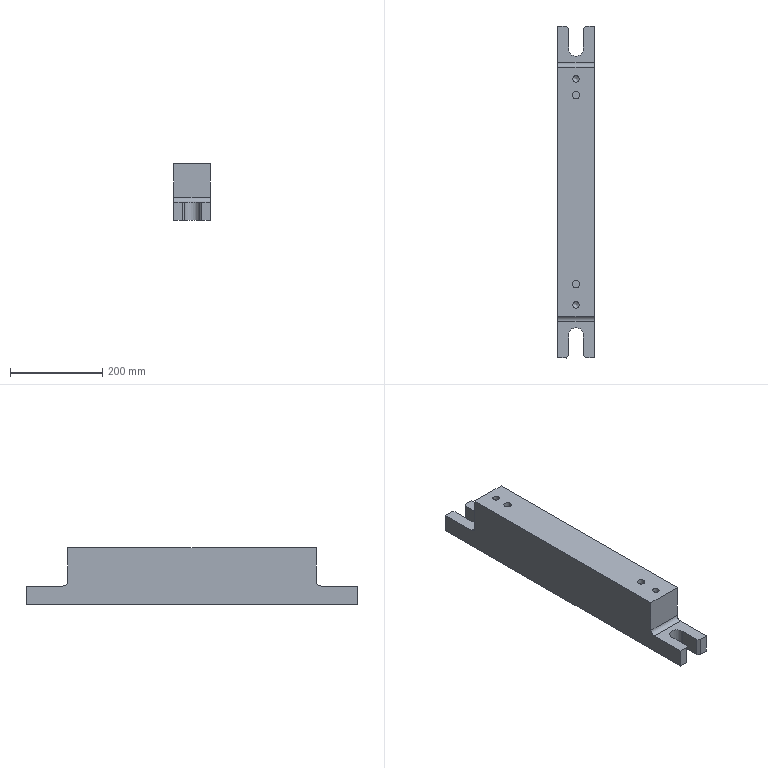Part | NX | features LIN_SOLID_COLOR 2 | 1 solid | 32 faces | box 80 x 720 x 123.5 mm | volume 5723645 mm3 | plane 22 | cylinder 8 | cone 2 | commonest cylinder face diameters 14 x2 16.002 x2 20 x2 32 x2
STEP:
#1=CARTESIAN_POINT('',(866.,-270.,-180.));
#2=VERTEX_POINT('',#1);
#3=CARTESIAN_POINT('',(786.,-270.,-180.));
#4=VERTEX_POINT('',#3);
#5=CARTESIAN_POINT('',(786.,-270.,-180.));
#6=DIRECTION('',(1.,0.,0.));
#7=VECTOR('',#6,1000.);
#8=LINE('',#5,#7);
#9=EDGE_CURVE('',#2,#4,#8,.F.);
#10=ORIENTED_EDGE('',*,*,#9,.F.);
#11=CARTESIAN_POINT('',(866.,-270.,-106.5));
#12=VERTEX_POINT('',#11);
#13=CARTESIAN_POINT('',(866.,-270.,-101.5));
#14=DIRECTION('',(0.,0.,-1.));
#15=VECTOR('',#14,1000.);
#16=LINE('',#13,#15);
#17=EDGE_CURVE('',#2,#12,#16,.F.);
#18=ORIENTED_EDGE('',*,*,#17,.T.);
#19=CARTESIAN_POINT('',(786.,-270.,-106.5));
#20=VERTEX_POINT('',#19);
#21=CARTESIAN_POINT('',(76.,-270.,-106.5));
#22=DIRECTION('',(1.,0.,0.));
#23=VECTOR('',#22,1000.);
#24=LINE('',#21,#23);
#25=EDGE_CURVE('',#12,#20,#24,.F.);
#26=ORIENTED_EDGE('',*,*,#25,.T.);
#27=CARTESIAN_POINT('',(786.,-270.,-101.5));
#28=DIRECTION('',(0.,0.,-1.));
#29=VECTOR('',#28,1000.);
#30=LINE('',#27,#29);
#31=EDGE_CURVE('',#4,#20,#30,.F.);
#32=ORIENTED_EDGE('',*,*,#31,.F.);
#33=EDGE_LOOP('',(#10,#18,#26,#32));
#34=FACE_BOUND('',#33,.T.);
#35=CARTESIAN_POINT('',(806.,-270.,-101.5));
#36=DIRECTION('',(0.,-1.,0.));
#37=DIRECTION('',(0.,0.,1.));
#38=AXIS2_PLACEMENT_3D('',#35,#36,#37);
#39=PLANE('',#38);
#40=ADVANCED_FACE('',(#34),#39,.T.);
#41=CARTESIAN_POINT('',(805.,-360.,-230.));
#42=VERTEX_POINT('',#41);
#43=CARTESIAN_POINT('',(786.,-360.,-230.));
#44=VERTEX_POINT('',#43);
#45=CARTESIAN_POINT('',(116.,-360.,-230.));
#46=DIRECTION('',(-1.,0.,0.));
#47=VECTOR('',#46,1000.);
#48=LINE('',#45,#47);
#49=EDGE_CURVE('',#42,#44,#48,.T.);
#50=ORIENTED_EDGE('',*,*,#49,.T.);
#51=CARTESIAN_POINT('',(786.,360.,-230.));
#52=VERTEX_POINT('',#51);
#53=CARTESIAN_POINT('',(786.,0.,-230.));
#54=DIRECTION('',(0.,-1.,0.));
#55=VECTOR('',#54,1000.);
#56=LINE('',#53,#55);
#57=EDGE_CURVE('',#52,#44,#56,.T.);
#58=ORIENTED_EDGE('',*,*,#57,.F.);
#59=CARTESIAN_POINT('',(805.,360.,-230.));
#60=VERTEX_POINT('',#59);
#61=CARTESIAN_POINT('',(116.,360.,-230.));
#62=DIRECTION('',(-1.,0.,0.));
#63=VECTOR('',#62,1000.);
#64=LINE('',#61,#63);
#65=EDGE_CURVE('',#60,#52,#64,.T.);
#66=ORIENTED_EDGE('',*,*,#65,.F.);
#67=CARTESIAN_POINT('',(810.,355.,-230.));
#68=VERTEX_POINT('',#67);
#69=CARTESIAN_POINT('',(126696.583,-125531.583,-230.));
#70=DIRECTION('',(0.7071,-0.7071,0.));
#71=VECTOR('',#70,1000.);
#72=LINE('',#69,#71);
#73=EDGE_CURVE('',#60,#68,#72,.T.);
#74=ORIENTED_EDGE('',*,*,#73,.T.);
#75=CARTESIAN_POINT('',(810.,310.,-230.));
#76=VERTEX_POINT('',#75);
#77=CARTESIAN_POINT('',(810.,1858.277,-230.));
#78=DIRECTION('',(0.,1.,0.));
#79=VECTOR('',#78,1000.);
#80=LINE('',#77,#79);
#81=EDGE_CURVE('',#76,#68,#80,.T.);
#82=ORIENTED_EDGE('',*,*,#81,.F.);
#83=CARTESIAN_POINT('',(842.,310.,-230.));
#84=VERTEX_POINT('',#83);
#85=CARTESIAN_POINT('',(826.,310.,-230.));
#86=DIRECTION('',(0.,0.,-1.));
#87=DIRECTION('',(1.,0.,0.));
#88=AXIS2_PLACEMENT_3D('',#85,#86,#87);
#89=CIRCLE('',#88,16.);
#90=EDGE_CURVE('',#84,#76,#89,.T.);
#91=ORIENTED_EDGE('',*,*,#90,.F.);
#92=CARTESIAN_POINT('',(842.,355.,-230.));
#93=VERTEX_POINT('',#92);
#94=CARTESIAN_POINT('',(842.,1858.277,-230.));
#95=DIRECTION('',(0.,-1.,0.));
#96=VECTOR('',#95,1000.);
#97=LINE('',#94,#96);
#98=EDGE_CURVE('',#93,#84,#97,.T.);
#99=ORIENTED_EDGE('',*,*,#98,.F.);
#100=CARTESIAN_POINT('',(847.,360.,-230.));
#101=VERTEX_POINT('',#100);
#102=CARTESIAN_POINT('',(128215.859,127728.859,-230.));
#103=DIRECTION('',(0.7071,0.7071,0.));
#104=VECTOR('',#103,1000.);
#105=LINE('',#102,#104);
#106=EDGE_CURVE('',#93,#101,#105,.T.);
#107=ORIENTED_EDGE('',*,*,#106,.T.);
#108=CARTESIAN_POINT('',(866.,360.,-230.));
#109=VERTEX_POINT('',#108);
#110=CARTESIAN_POINT('',(116.,360.,-230.));
#111=DIRECTION('',(-1.,0.,0.));
#112=VECTOR('',#111,1000.);
#113=LINE('',#110,#112);
#114=EDGE_CURVE('',#109,#101,#113,.T.);
#115=ORIENTED_EDGE('',*,*,#114,.F.);
#116=CARTESIAN_POINT('',(866.,-360.,-230.));
#117=VERTEX_POINT('',#116);
#118=CARTESIAN_POINT('',(866.,0.,-230.));
#119=DIRECTION('',(0.,-1.,0.));
#120=VECTOR('',#119,1000.);
#121=LINE('',#118,#120);
#122=EDGE_CURVE('',#109,#117,#121,.T.);
#123=ORIENTED_EDGE('',*,*,#122,.T.);
#124=CARTESIAN_POINT('',(847.,-360.,-230.));
#125=VERTEX_POINT('',#124);
#126=CARTESIAN_POINT('',(116.,-360.,-230.));
#127=DIRECTION('',(-1.,0.,0.));
#128=VECTOR('',#127,1000.);
#129=LINE('',#126,#128);
#130=EDGE_CURVE('',#117,#125,#129,.T.);
#131=ORIENTED_EDGE('',*,*,#130,.T.);
#132=CARTESIAN_POINT('',(842.,-355.,-230.));
#133=VERTEX_POINT('',#132);
#134=CARTESIAN_POINT('',(128215.859,-127728.859,-230.));
#135=DIRECTION('',(0.7071,-0.7071,0.));
#136=VECTOR('',#135,1000.);
#137=LINE('',#134,#136);
#138=EDGE_CURVE('',#133,#125,#137,.T.);
#139=ORIENTED_EDGE('',*,*,#138,.F.);
#140=CARTESIAN_POINT('',(842.,-310.,-230.));
#141=VERTEX_POINT('',#140);
#142=CARTESIAN_POINT('',(842.,-1858.277,-230.));
#143=DIRECTION('',(0.,1.,0.));
#144=VECTOR('',#143,1000.);
#145=LINE('',#142,#144);
#146=EDGE_CURVE('',#133,#141,#145,.T.);
#147=ORIENTED_EDGE('',*,*,#146,.T.);
#148=CARTESIAN_POINT('',(810.,-310.,-230.));
#149=VERTEX_POINT('',#148);
#150=CARTESIAN_POINT('',(826.,-310.,-230.));
#151=DIRECTION('',(0.,0.,1.));
#152=DIRECTION('',(1.,0.,0.));
#153=AXIS2_PLACEMENT_3D('',#150,#151,#152);
#154=CIRCLE('',#153,16.);
#155=EDGE_CURVE('',#141,#149,#154,.T.);
#156=ORIENTED_EDGE('',*,*,#155,.T.);
#157=CARTESIAN_POINT('',(810.,-355.,-230.));
#158=VERTEX_POINT('',#157);
#159=CARTESIAN_POINT('',(810.,-1858.277,-230.));
#160=DIRECTION('',(0.,-1.,0.));
#161=VECTOR('',#160,1000.);
#162=LINE('',#159,#161);
#163=EDGE_CURVE('',#149,#158,#162,.T.);
#164=ORIENTED_EDGE('',*,*,#163,.T.);
#165=CARTESIAN_POINT('',(126696.583,125531.583,-230.));
#166=DIRECTION('',(0.7071,0.7071,0.));
#167=VECTOR('',#166,1000.);
#168=LINE('',#165,#167);
#169=EDGE_CURVE('',#42,#158,#168,.T.);
#170=ORIENTED_EDGE('',*,*,#169,.F.);
#171=EDGE_LOOP('',(#50,#58,#66,#74,#82,#91,#99,#107,#115,#123,#131,#139,#147,#156,#164,#170));
#172=FACE_BOUND('',#171,.T.);
#173=CARTESIAN_POINT('',(666.,0.,-230.));
#174=DIRECTION('',(0.,0.,1.));
#175=DIRECTION('',(-1.,0.,0.));
#176=AXIS2_PLACEMENT_3D('',#173,#174,#175);
#177=PLANE('',#176);
#178=ADVANCED_FACE('',(#172),#177,.F.);
#179=CARTESIAN_POINT('',(866.,270.,-106.5));
#180=VERTEX_POINT('',#179);
#181=CARTESIAN_POINT('',(866.,0.,-106.5));
#182=DIRECTION('',(0.,1.,0.));
#183=VECTOR('',#182,1000.);
#184=LINE('',#181,#183);
#185=EDGE_CURVE('',#12,#180,#184,.T.);
#186=ORIENTED_EDGE('',*,*,#185,.T.);
#187=CARTESIAN_POINT('',(786.,270.,-106.5));
#188=VERTEX_POINT('',#187);
#189=CARTESIAN_POINT('',(806.,270.,-106.5));
#190=DIRECTION('',(-1.,0.,0.));
#191=VECTOR('',#190,1000.);
#192=LINE('',#189,#191);
#193=EDGE_CURVE('',#180,#188,#192,.T.);
#194=ORIENTED_EDGE('',*,*,#193,.T.);
#195=CARTESIAN_POINT('',(786.,0.,-106.5));
#196=DIRECTION('',(0.,1.,0.));
#197=VECTOR('',#196,1000.);
#198=LINE('',#195,#197);
#199=EDGE_CURVE('',#20,#188,#198,.T.);
#200=ORIENTED_EDGE('',*,*,#199,.F.);
#201=ORIENTED_EDGE('',*,*,#25,.F.);
#202=EDGE_LOOP('',(#186,#194,#200,#201));
#203=FACE_BOUND('',#202,.T.);
#204=CARTESIAN_POINT('',(817.999,210.,-106.5));
#205=VERTEX_POINT('',#204);
#206=CARTESIAN_POINT('',(826.,210.,-106.5));
#207=DIRECTION('',(0.,0.,-1.));
#208=DIRECTION('',(-1.,0.,0.));
#209=AXIS2_PLACEMENT_3D('',#206,#207,#208);
#210=CIRCLE('',#209,8.001);
#211=EDGE_CURVE('',#205,#205,#210,.T.);
#212=ORIENTED_EDGE('',*,*,#211,.T.);
#213=EDGE_LOOP('',(#212));
#214=FACE_BOUND('',#213,.T.);
#215=CARTESIAN_POINT('',(819.,-245.,-106.5));
#216=VERTEX_POINT('',#215);
#217=CARTESIAN_POINT('',(826.,-245.,-106.5));
#218=DIRECTION('',(0.,0.,-1.));
#219=DIRECTION('',(-1.,0.,0.));
#220=AXIS2_PLACEMENT_3D('',#217,#218,#219);
#221=CIRCLE('',#220,7.);
#222=EDGE_CURVE('',#216,#216,#221,.T.);
#223=ORIENTED_EDGE('',*,*,#222,.T.);
#224=EDGE_LOOP('',(#223));
#225=FACE_BOUND('',#224,.T.);
#226=CARTESIAN_POINT('',(819.,245.,-106.5));
#227=VERTEX_POINT('',#226);
#228=CARTESIAN_POINT('',(826.,245.,-106.5));
#229=DIRECTION('',(0.,0.,-1.));
#230=DIRECTION('',(-1.,0.,0.));
#231=AXIS2_PLACEMENT_3D('',#228,#229,#230);
#232=CIRCLE('',#231,7.);
#233=EDGE_CURVE('',#227,#227,#232,.T.);
#234=ORIENTED_EDGE('',*,*,#233,.T.);
#235=EDGE_LOOP('',(#234));
#236=FACE_BOUND('',#235,.T.);
#237=CARTESIAN_POINT('',(817.999,-200.,-106.5));
#238=VERTEX_POINT('',#237);
#239=CARTESIAN_POINT('',(826.,-200.,-106.5));
#240=DIRECTION('',(0.,0.,-1.));
#241=DIRECTION('',(-1.,0.,0.));
#242=AXIS2_PLACEMENT_3D('',#239,#240,#241);
#243=CIRCLE('',#242,8.001);
#244=EDGE_CURVE('',#238,#238,#243,.F.);
#245=ORIENTED_EDGE('',*,*,#244,.F.);
#246=EDGE_LOOP('',(#245));
#247=FACE_BOUND('',#246,.T.);
#248=CARTESIAN_POINT('',(76.,0.,-106.5));
#249=DIRECTION('',(0.,0.,-1.));
#250=DIRECTION('',(1.,0.,0.));
#251=AXIS2_PLACEMENT_3D('',#248,#249,#250);
#252=PLANE('',#251);
#253=ADVANCED_FACE('',(#203,#214,#225,#236,#247),#252,.F.);
#254=CARTESIAN_POINT('',(866.,270.,-180.));
#255=VERTEX_POINT('',#254);
#256=CARTESIAN_POINT('',(866.,270.,-101.5));
#257=DIRECTION('',(0.,0.,1.));
#258=VECTOR('',#257,1000.);
#259=LINE('',#256,#258);
#260=EDGE_CURVE('',#255,#180,#259,.T.);
#261=ORIENTED_EDGE('',*,*,#260,.F.);
#262=CARTESIAN_POINT('',(786.,270.,-180.));
#263=VERTEX_POINT('',#262);
#264=CARTESIAN_POINT('',(786.,270.,-180.));
#265=DIRECTION('',(1.,0.,0.));
#266=VECTOR('',#265,1000.);
#267=LINE('',#264,#266);
#268=EDGE_CURVE('',#255,#263,#267,.F.);
#269=ORIENTED_EDGE('',*,*,#268,.T.);
#270=CARTESIAN_POINT('',(786.,270.,-101.5));
#271=DIRECTION('',(0.,0.,1.));
#272=VECTOR('',#271,1000.);
#273=LINE('',#270,#272);
#274=EDGE_CURVE('',#263,#188,#273,.T.);
#275=ORIENTED_EDGE('',*,*,#274,.T.);
#276=ORIENTED_EDGE('',*,*,#193,.F.);
#277=EDGE_LOOP('',(#261,#269,#275,#276));
#278=FACE_BOUND('',#277,.T.);
#279=CARTESIAN_POINT('',(806.,270.,-101.5));
#280=DIRECTION('',(0.,-1.,0.));
#281=DIRECTION('',(0.,0.,1.));
#282=AXIS2_PLACEMENT_3D('',#279,#280,#281);
#283=PLANE('',#282);
#284=ADVANCED_FACE('',(#278),#283,.F.);
#285=ORIENTED_EDGE('',*,*,#199,.T.);
#286=ORIENTED_EDGE('',*,*,#274,.F.);
#287=CARTESIAN_POINT('',(786.,280.,-190.));
#288=VERTEX_POINT('',#287);
#289=CARTESIAN_POINT('',(786.,280.,-180.));
#290=DIRECTION('',(1.,0.,0.));
#291=DIRECTION('',(0.,0.,1.));
#292=AXIS2_PLACEMENT_3D('',#289,#290,#291);
#293=CIRCLE('',#292,10.);
#294=EDGE_CURVE('',#263,#288,#293,.T.);
#295=ORIENTED_EDGE('',*,*,#294,.T.);
#296=CARTESIAN_POINT('',(786.,360.,-190.));
#297=VERTEX_POINT('',#296);
#298=CARTESIAN_POINT('',(786.,320.,-190.));
#299=DIRECTION('',(0.,1.,0.));
#300=VECTOR('',#299,1000.);
#301=LINE('',#298,#300);
#302=EDGE_CURVE('',#288,#297,#301,.T.);
#303=ORIENTED_EDGE('',*,*,#302,.T.);
#304=CARTESIAN_POINT('',(786.,360.,-131.5));
#305=DIRECTION('',(0.,0.,1.));
#306=VECTOR('',#305,1000.);
#307=LINE('',#304,#306);
#308=EDGE_CURVE('',#52,#297,#307,.T.);
#309=ORIENTED_EDGE('',*,*,#308,.F.);
#310=ORIENTED_EDGE('',*,*,#57,.T.);
#311=CARTESIAN_POINT('',(786.,-360.,-190.));
#312=VERTEX_POINT('',#311);
#313=CARTESIAN_POINT('',(786.,-360.,-131.5));
#314=DIRECTION('',(0.,0.,1.));
#315=VECTOR('',#314,1000.);
#316=LINE('',#313,#315);
#317=EDGE_CURVE('',#44,#312,#316,.T.);
#318=ORIENTED_EDGE('',*,*,#317,.T.);
#319=CARTESIAN_POINT('',(786.,-280.,-190.));
#320=VERTEX_POINT('',#319);
#321=CARTESIAN_POINT('',(786.,-320.,-190.));
#322=DIRECTION('',(0.,-1.,0.));
#323=VECTOR('',#322,1000.);
#324=LINE('',#321,#323);
#325=EDGE_CURVE('',#320,#312,#324,.T.);
#326=ORIENTED_EDGE('',*,*,#325,.F.);
#327=CARTESIAN_POINT('',(786.,-280.,-180.));
#328=DIRECTION('',(-1.,0.,0.));
#329=DIRECTION('',(0.,0.,1.));
#330=AXIS2_PLACEMENT_3D('',#327,#328,#329);
#331=CIRCLE('',#330,10.);
#332=EDGE_CURVE('',#4,#320,#331,.T.);
#333=ORIENTED_EDGE('',*,*,#332,.F.);
#334=ORIENTED_EDGE('',*,*,#31,.T.);
#335=EDGE_LOOP('',(#285,#286,#295,#303,#309,#310,#318,#326,#333,#334));
#336=FACE_BOUND('',#335,.T.);
#337=CARTESIAN_POINT('',(786.,0.,-101.5));
#338=DIRECTION('',(1.,0.,0.));
#339=DIRECTION('',(0.,0.,1.));
#340=AXIS2_PLACEMENT_3D('',#337,#338,#339);
#341=PLANE('',#340);
#342=ADVANCED_FACE('',(#336),#341,.F.);
#343=CARTESIAN_POINT('',(866.,-360.,-190.));
#344=VERTEX_POINT('',#343);
#345=CARTESIAN_POINT('',(866.,-360.,-111.5));
#346=DIRECTION('',(0.,0.,1.));
#347=VECTOR('',#346,1000.);
#348=LINE('',#345,#347);
#349=EDGE_CURVE('',#117,#344,#348,.T.);
#350=ORIENTED_EDGE('',*,*,#349,.F.);
#351=ORIENTED_EDGE('',*,*,#122,.F.);
#352=CARTESIAN_POINT('',(866.,360.,-190.));
#353=VERTEX_POINT('',#352);
#354=CARTESIAN_POINT('',(866.,360.,-111.5));
#355=DIRECTION('',(0.,0.,1.));
#356=VECTOR('',#355,1000.);
#357=LINE('',#354,#356);
#358=EDGE_CURVE('',#109,#353,#357,.T.);
#359=ORIENTED_EDGE('',*,*,#358,.T.);
#360=CARTESIAN_POINT('',(866.,280.,-190.));
#361=VERTEX_POINT('',#360);
#362=CARTESIAN_POINT('',(866.,10.,-190.));
#363=DIRECTION('',(0.,-1.,0.));
#364=VECTOR('',#363,1000.);
#365=LINE('',#362,#364);
#366=EDGE_CURVE('',#353,#361,#365,.T.);
#367=ORIENTED_EDGE('',*,*,#366,.T.);
#368=CARTESIAN_POINT('',(866.,280.,-180.));
#369=DIRECTION('',(1.,0.,0.));
#370=DIRECTION('',(0.,0.,1.));
#371=AXIS2_PLACEMENT_3D('',#368,#369,#370);
#372=CIRCLE('',#371,10.);
#373=EDGE_CURVE('',#361,#255,#372,.F.);
#374=ORIENTED_EDGE('',*,*,#373,.T.);
#375=ORIENTED_EDGE('',*,*,#260,.T.);
#376=ORIENTED_EDGE('',*,*,#185,.F.);
#377=ORIENTED_EDGE('',*,*,#17,.F.);
#378=CARTESIAN_POINT('',(866.,-280.,-190.));
#379=VERTEX_POINT('',#378);
#380=CARTESIAN_POINT('',(866.,-280.,-180.));
#381=DIRECTION('',(-1.,0.,0.));
#382=DIRECTION('',(0.,0.,1.));
#383=AXIS2_PLACEMENT_3D('',#380,#381,#382);
#384=CIRCLE('',#383,10.);
#385=EDGE_CURVE('',#379,#2,#384,.F.);
#386=ORIENTED_EDGE('',*,*,#385,.F.);
#387=CARTESIAN_POINT('',(866.,-10.,-190.));
#388=DIRECTION('',(0.,1.,0.));
#389=VECTOR('',#388,1000.);
#390=LINE('',#387,#389);
#391=EDGE_CURVE('',#344,#379,#390,.T.);
#392=ORIENTED_EDGE('',*,*,#391,.F.);
#393=EDGE_LOOP('',(#350,#351,#359,#367,#374,#375,#376,#377,#386,#392));
#394=FACE_BOUND('',#393,.T.);
#395=CARTESIAN_POINT('',(866.,0.,-101.5));
#396=DIRECTION('',(1.,0.,0.));
#397=DIRECTION('',(0.,0.,1.));
#398=AXIS2_PLACEMENT_3D('',#395,#396,#397);
#399=PLANE('',#398);
#400=ADVANCED_FACE('',(#394),#399,.T.);
#401=CARTESIAN_POINT('',(833.,-245.,-146.5));
#402=VERTEX_POINT('',#401);
#403=CARTESIAN_POINT('',(826.,-245.,-146.5));
#404=DIRECTION('',(0.,0.,1.));
#405=DIRECTION('',(1.,0.,0.));
#406=AXIS2_PLACEMENT_3D('',#403,#404,#405);
#407=CIRCLE('',#406,7.);
#408=EDGE_CURVE('',#402,#402,#407,.T.);
#409=ORIENTED_EDGE('',*,*,#408,.F.);
#410=EDGE_LOOP('',(#409));
#411=FACE_BOUND('',#410,.T.);
#412=ORIENTED_EDGE('',*,*,#222,.F.);
#413=EDGE_LOOP('',(#412));
#414=FACE_BOUND('',#413,.T.);
#415=CARTESIAN_POINT('',(826.,-245.,-106.4));
#416=DIRECTION('',(0.,0.,-1.));
#417=DIRECTION('',(1.,0.,0.));
#418=AXIS2_PLACEMENT_3D('',#415,#416,#417);
#419=CYLINDRICAL_SURFACE('',#418,7.);
#420=ADVANCED_FACE('',(#411,#414),#419,.F.);
#421=ORIENTED_EDGE('',*,*,#408,.T.);
#422=EDGE_LOOP('',(#421));
#423=FACE_BOUND('',#422,.T.);
#424=CARTESIAN_POINT('',(826.,-245.,-150.541));
#425=VERTEX_POINT('',#424);
#426=VERTEX_LOOP('',#425);
#427=FACE_BOUND('',#426,.T.);
#428=CARTESIAN_POINT('',(826.,-245.,-150.541));
#429=DIRECTION('',(0.,0.,1.));
#430=DIRECTION('',(1.,0.,0.));
#431=AXIS2_PLACEMENT_3D('',#428,#429,#430);
#432=CONICAL_SURFACE('',#431,0.,1.047);
#433=ADVANCED_FACE('',(#423,#427),#432,.F.);
#434=CARTESIAN_POINT('',(833.,245.,-146.5));
#435=VERTEX_POINT('',#434);
#436=CARTESIAN_POINT('',(826.,245.,-146.5));
#437=DIRECTION('',(0.,0.,1.));
#438=DIRECTION('',(1.,0.,0.));
#439=AXIS2_PLACEMENT_3D('',#436,#437,#438);
#440=CIRCLE('',#439,7.);
#441=EDGE_CURVE('',#435,#435,#440,.T.);
#442=ORIENTED_EDGE('',*,*,#441,.F.);
#443=EDGE_LOOP('',(#442));
#444=FACE_BOUND('',#443,.T.);
#445=ORIENTED_EDGE('',*,*,#233,.F.);
#446=EDGE_LOOP('',(#445));
#447=FACE_BOUND('',#446,.T.);
#448=CARTESIAN_POINT('',(826.,245.,-106.4));
#449=DIRECTION('',(0.,0.,-1.));
#450=DIRECTION('',(1.,0.,0.));
#451=AXIS2_PLACEMENT_3D('',#448,#449,#450);
#452=CYLINDRICAL_SURFACE('',#451,7.);
#453=ADVANCED_FACE('',(#444,#447),#452,.F.);
#454=ORIENTED_EDGE('',*,*,#441,.T.);
#455=EDGE_LOOP('',(#454));
#456=FACE_BOUND('',#455,.T.);
#457=CARTESIAN_POINT('',(826.,245.,-150.541));
#458=VERTEX_POINT('',#457);
#459=VERTEX_LOOP('',#458);
#460=FACE_BOUND('',#459,.T.);
#461=CARTESIAN_POINT('',(826.,245.,-150.541));
#462=DIRECTION('',(0.,0.,1.));
#463=DIRECTION('',(1.,0.,0.));
#464=AXIS2_PLACEMENT_3D('',#461,#462,#463);
#465=CONICAL_SURFACE('',#464,0.,1.047);
#466=ADVANCED_FACE('',(#456,#460),#465,.F.);
#467=CARTESIAN_POINT('',(834.001,-200.,-146.5));
#468=VERTEX_POINT('',#467);
#469=CARTESIAN_POINT('',(826.,-200.,-146.5));
#470=DIRECTION('',(0.,0.,1.));
#471=DIRECTION('',(1.,0.,0.));
#472=AXIS2_PLACEMENT_3D('',#469,#470,#471);
#473=CIRCLE('',#472,8.001);
#474=EDGE_CURVE('',#468,#468,#473,.T.);
#475=ORIENTED_EDGE('',*,*,#474,.F.);
#476=EDGE_LOOP('',(#475));
#477=FACE_BOUND('',#476,.T.);
#478=ORIENTED_EDGE('',*,*,#244,.T.);
#479=EDGE_LOOP('',(#478));
#480=FACE_BOUND('',#479,.T.);
#481=CARTESIAN_POINT('',(826.,-200.,-304.5));
#482=DIRECTION('',(0.,0.,1.));
#483=DIRECTION('',(1.,0.,0.));
#484=AXIS2_PLACEMENT_3D('',#481,#482,#483);
#485=CYLINDRICAL_SURFACE('',#484,8.001);
#486=ADVANCED_FACE('',(#477,#480),#485,.F.);
#487=CARTESIAN_POINT('',(834.001,210.,-146.5));
#488=VERTEX_POINT('',#487);
#489=CARTESIAN_POINT('',(826.,210.,-146.5));
#490=DIRECTION('',(0.,0.,1.));
#491=DIRECTION('',(1.,0.,0.));
#492=AXIS2_PLACEMENT_3D('',#489,#490,#491);
#493=CIRCLE('',#492,8.001);
#494=EDGE_CURVE('',#488,#488,#493,.T.);
#495=ORIENTED_EDGE('',*,*,#494,.F.);
#496=EDGE_LOOP('',(#495));
#497=FACE_BOUND('',#496,.T.);
#498=ORIENTED_EDGE('',*,*,#211,.F.);
#499=EDGE_LOOP('',(#498));
#500=FACE_BOUND('',#499,.T.);
#501=CARTESIAN_POINT('',(826.,210.,-304.5));
#502=DIRECTION('',(0.,0.,1.));
#503=DIRECTION('',(1.,0.,0.));
#504=AXIS2_PLACEMENT_3D('',#501,#502,#503);
#505=CYLINDRICAL_SURFACE('',#504,8.001);
#506=ADVANCED_FACE('',(#497,#500),#505,.F.);
#507=ORIENTED_EDGE('',*,*,#130,.F.);
#508=ORIENTED_EDGE('',*,*,#349,.T.);
#509=CARTESIAN_POINT('',(847.,-360.,-190.));
#510=VERTEX_POINT('',#509);
#511=CARTESIAN_POINT('',(116.,-360.,-190.));
#512=DIRECTION('',(1.,0.,0.));
#513=VECTOR('',#512,1000.);
#514=LINE('',#511,#513);
#515=EDGE_CURVE('',#510,#344,#514,.T.);
#516=ORIENTED_EDGE('',*,*,#515,.F.);
#517=CARTESIAN_POINT('',(847.,-360.,-200.));
#518=DIRECTION('',(0.,0.,1.));
#519=VECTOR('',#518,1000.);
#520=LINE('',#517,#519);
#521=EDGE_CURVE('',#125,#510,#520,.T.);
#522=ORIENTED_EDGE('',*,*,#521,.F.);
#523=EDGE_LOOP('',(#507,#508,#516,#522));
#524=FACE_BOUND('',#523,.T.);
#525=CARTESIAN_POINT('',(116.,-360.,-131.5));
#526=DIRECTION('',(0.,-1.,0.));
#527=DIRECTION('',(0.,0.,-1.));
#528=AXIS2_PLACEMENT_3D('',#525,#526,#527);
#529=PLANE('',#528);
#530=ADVANCED_FACE('',(#524),#529,.T.);
#531=ORIENTED_EDGE('',*,*,#138,.T.);
#532=ORIENTED_EDGE('',*,*,#521,.T.);
#533=CARTESIAN_POINT('',(842.,-355.,-190.));
#534=VERTEX_POINT('',#533);
#535=CARTESIAN_POINT('',(616.5,-129.5,-190.));
#536=DIRECTION('',(-0.7071,0.7071,0.));
#537=VECTOR('',#536,1000.);
#538=LINE('',#535,#537);
#539=EDGE_CURVE('',#510,#534,#538,.T.);
#540=ORIENTED_EDGE('',*,*,#539,.T.);
#541=CARTESIAN_POINT('',(842.,-355.,-230.));
#542=DIRECTION('',(0.,0.,-1.));
#543=VECTOR('',#542,1000.);
#544=LINE('',#541,#543);
#545=EDGE_CURVE('',#534,#133,#544,.T.);
#546=ORIENTED_EDGE('',*,*,#545,.T.);
#547=EDGE_LOOP('',(#531,#532,#540,#546));
#548=FACE_BOUND('',#547,.T.);
#549=CARTESIAN_POINT('',(847.,-360.,-131.5));
#550=DIRECTION('',(-0.7071,-0.7071,0.));
#551=DIRECTION('',(0.,0.,-1.));
#552=AXIS2_PLACEMENT_3D('',#549,#550,#551);
#553=PLANE('',#552);
#554=ADVANCED_FACE('',(#548),#553,.T.);
#555=CARTESIAN_POINT('',(842.,-310.,-190.));
#556=VERTEX_POINT('',#555);
#557=CARTESIAN_POINT('',(842.,-30.,-190.));
#558=DIRECTION('',(0.,-1.,0.));
#559=VECTOR('',#558,1000.);
#560=LINE('',#557,#559);
#561=EDGE_CURVE('',#556,#534,#560,.T.);
#562=ORIENTED_EDGE('',*,*,#561,.F.);
#563=CARTESIAN_POINT('',(842.,-310.,-305.));
#564=DIRECTION('',(0.,0.,1.));
#565=VECTOR('',#564,1000.);
#566=LINE('',#563,#565);
#567=EDGE_CURVE('',#556,#141,#566,.F.);
#568=ORIENTED_EDGE('',*,*,#567,.T.);
#569=ORIENTED_EDGE('',*,*,#146,.F.);
#570=ORIENTED_EDGE('',*,*,#545,.F.);
#571=EDGE_LOOP('',(#562,#568,#569,#570));
#572=FACE_BOUND('',#571,.T.);
#573=CARTESIAN_POINT('',(842.,-60.,-305.));
#574=DIRECTION('',(1.,0.,0.));
#575=DIRECTION('',(0.,0.,1.));
#576=AXIS2_PLACEMENT_3D('',#573,#574,#575);
#577=PLANE('',#576);
#578=ADVANCED_FACE('',(#572),#577,.F.);
#579=CARTESIAN_POINT('',(810.,-310.,-190.));
#580=VERTEX_POINT('',#579);
#581=CARTESIAN_POINT('',(826.,-310.,-190.));
#582=DIRECTION('',(0.,0.,-1.));
#583=DIRECTION('',(-1.,0.,0.));
#584=AXIS2_PLACEMENT_3D('',#581,#582,#583);
#585=CIRCLE('',#584,16.);
#586=EDGE_CURVE('',#580,#556,#585,.T.);
#587=ORIENTED_EDGE('',*,*,#586,.F.);
#588=CARTESIAN_POINT('',(810.,-310.,-305.));
#589=DIRECTION('',(0.,0.,-1.));
#590=VECTOR('',#589,1000.);
#591=LINE('',#588,#590);
#592=EDGE_CURVE('',#149,#580,#591,.F.);
#593=ORIENTED_EDGE('',*,*,#592,.F.);
#594=ORIENTED_EDGE('',*,*,#155,.F.);
#595=ORIENTED_EDGE('',*,*,#567,.F.);
#596=EDGE_LOOP('',(#587,#593,#594,#595));
#597=FACE_BOUND('',#596,.T.);
#598=CARTESIAN_POINT('',(826.,-310.,-155.));
#599=DIRECTION('',(0.,0.,-1.));
#600=DIRECTION('',(1.,0.,0.));
#601=AXIS2_PLACEMENT_3D('',#598,#599,#600);
#602=CYLINDRICAL_SURFACE('',#601,16.);
#603=ADVANCED_FACE('',(#597),#602,.F.);
#604=ORIENTED_EDGE('',*,*,#163,.F.);
#605=ORIENTED_EDGE('',*,*,#592,.T.);
#606=CARTESIAN_POINT('',(810.,-355.,-190.));
#607=VERTEX_POINT('',#606);
#608=CARTESIAN_POINT('',(810.,-30.,-190.));
#609=DIRECTION('',(0.,1.,0.));
#610=VECTOR('',#609,1000.);
#611=LINE('',#608,#610);
#612=EDGE_CURVE('',#607,#580,#611,.T.);
#613=ORIENTED_EDGE('',*,*,#612,.F.);
#614=CARTESIAN_POINT('',(810.,-355.,-200.));
#615=DIRECTION('',(0.,0.,1.));
#616=VECTOR('',#615,1000.);
#617=LINE('',#614,#616);
#618=EDGE_CURVE('',#158,#607,#617,.T.);
#619=ORIENTED_EDGE('',*,*,#618,.F.);
#620=EDGE_LOOP('',(#604,#605,#613,#619));
#621=FACE_BOUND('',#620,.T.);
#622=CARTESIAN_POINT('',(810.,-60.,-305.));
#623=DIRECTION('',(-1.,0.,0.));
#624=DIRECTION('',(0.,0.,-1.));
#625=AXIS2_PLACEMENT_3D('',#622,#623,#624);
#626=PLANE('',#625);
#627=ADVANCED_FACE('',(#621),#626,.F.);
#628=ORIENTED_EDGE('',*,*,#169,.T.);
#629=ORIENTED_EDGE('',*,*,#618,.T.);
#630=CARTESIAN_POINT('',(805.,-360.,-190.));
#631=VERTEX_POINT('',#630);
#632=CARTESIAN_POINT('',(925.5,-239.5,-190.));
#633=DIRECTION('',(-0.7071,-0.7071,0.));
#634=VECTOR('',#633,1000.);
#635=LINE('',#632,#634);
#636=EDGE_CURVE('',#607,#631,#635,.T.);
#637=ORIENTED_EDGE('',*,*,#636,.T.);
#638=CARTESIAN_POINT('',(805.,-360.,-230.));
#639=DIRECTION('',(0.,0.,-1.));
#640=VECTOR('',#639,1000.);
#641=LINE('',#638,#640);
#642=EDGE_CURVE('',#631,#42,#641,.T.);
#643=ORIENTED_EDGE('',*,*,#642,.T.);
#644=EDGE_LOOP('',(#628,#629,#637,#643));
#645=FACE_BOUND('',#644,.T.);
#646=CARTESIAN_POINT('',(810.,-355.,-305.));
#647=DIRECTION('',(0.7071,-0.7071,0.));
#648=DIRECTION('',(0.,0.,-1.));
#649=AXIS2_PLACEMENT_3D('',#646,#647,#648);
#650=PLANE('',#649);
#651=ADVANCED_FACE('',(#645),#650,.T.);
#652=ORIENTED_EDGE('',*,*,#49,.F.);
#653=ORIENTED_EDGE('',*,*,#642,.F.);
#654=CARTESIAN_POINT('',(116.,-360.,-190.));
#655=DIRECTION('',(1.,0.,0.));
#656=VECTOR('',#655,1000.);
#657=LINE('',#654,#656);
#658=EDGE_CURVE('',#312,#631,#657,.T.);
#659=ORIENTED_EDGE('',*,*,#658,.F.);
#660=ORIENTED_EDGE('',*,*,#317,.F.);
#661=EDGE_LOOP('',(#652,#653,#659,#660));
#662=FACE_BOUND('',#661,.T.);
#663=CARTESIAN_POINT('',(116.,-360.,-131.5));
#664=DIRECTION('',(0.,-1.,0.));
#665=DIRECTION('',(0.,0.,-1.));
#666=AXIS2_PLACEMENT_3D('',#663,#664,#665);
#667=PLANE('',#666);
#668=ADVANCED_FACE('',(#662),#667,.T.);
#669=ORIENTED_EDGE('',*,*,#325,.T.);
#670=ORIENTED_EDGE('',*,*,#658,.T.);
#671=ORIENTED_EDGE('',*,*,#636,.F.);
#672=ORIENTED_EDGE('',*,*,#612,.T.);
#673=ORIENTED_EDGE('',*,*,#586,.T.);
#674=ORIENTED_EDGE('',*,*,#561,.T.);
#675=ORIENTED_EDGE('',*,*,#539,.F.);
#676=ORIENTED_EDGE('',*,*,#515,.T.);
#677=ORIENTED_EDGE('',*,*,#391,.T.);
#678=CARTESIAN_POINT('',(866.,-280.,-190.));
#679=DIRECTION('',(1.,0.,0.));
#680=VECTOR('',#679,1000.);
#681=LINE('',#678,#680);
#682=EDGE_CURVE('',#320,#379,#681,.T.);
#683=ORIENTED_EDGE('',*,*,#682,.F.);
#684=EDGE_LOOP('',(#669,#670,#671,#672,#673,#674,#675,#676,#677,#683));
#685=FACE_BOUND('',#684,.T.);
#686=CARTESIAN_POINT('',(716.,-30.,-190.));
#687=DIRECTION('',(0.,0.,1.));
#688=DIRECTION('',(-1.,0.,0.));
#689=AXIS2_PLACEMENT_3D('',#686,#687,#688);
#690=PLANE('',#689);
#691=ADVANCED_FACE('',(#685),#690,.T.);
#692=ORIENTED_EDGE('',*,*,#332,.T.);
#693=ORIENTED_EDGE('',*,*,#682,.T.);
#694=ORIENTED_EDGE('',*,*,#385,.T.);
#695=ORIENTED_EDGE('',*,*,#9,.T.);
#696=EDGE_LOOP('',(#692,#693,#694,#695));
#697=FACE_BOUND('',#696,.T.);
#698=CARTESIAN_POINT('',(716.,-280.,-180.));
#699=DIRECTION('',(-1.,0.,0.));
#700=DIRECTION('',(0.,0.,-1.));
#701=AXIS2_PLACEMENT_3D('',#698,#699,#700);
#702=CYLINDRICAL_SURFACE('',#701,10.);
#703=ADVANCED_FACE('',(#697),#702,.F.);
#704=ORIENTED_EDGE('',*,*,#114,.T.);
#705=CARTESIAN_POINT('',(847.,360.,-190.));
#706=VERTEX_POINT('',#705);
#707=CARTESIAN_POINT('',(847.,360.,-200.));
#708=DIRECTION('',(0.,0.,1.));
#709=VECTOR('',#708,1000.);
#710=LINE('',#707,#709);
#711=EDGE_CURVE('',#101,#706,#710,.T.);
#712=ORIENTED_EDGE('',*,*,#711,.T.);
#713=CARTESIAN_POINT('',(116.,360.,-190.));
#714=DIRECTION('',(1.,0.,0.));
#715=VECTOR('',#714,1000.);
#716=LINE('',#713,#715);
#717=EDGE_CURVE('',#706,#353,#716,.T.);
#718=ORIENTED_EDGE('',*,*,#717,.T.);
#719=ORIENTED_EDGE('',*,*,#358,.F.);
#720=EDGE_LOOP('',(#704,#712,#718,#719));
#721=FACE_BOUND('',#720,.T.);
#722=CARTESIAN_POINT('',(116.,360.,-131.5));
#723=DIRECTION('',(0.,1.,0.));
#724=DIRECTION('',(0.,0.,-1.));
#725=AXIS2_PLACEMENT_3D('',#722,#723,#724);
#726=PLANE('',#725);
#727=ADVANCED_FACE('',(#721),#726,.T.);
#728=ORIENTED_EDGE('',*,*,#106,.F.);
#729=CARTESIAN_POINT('',(842.,355.,-190.));
#730=VERTEX_POINT('',#729);
#731=CARTESIAN_POINT('',(842.,355.,-230.));
#732=DIRECTION('',(0.,0.,-1.));
#733=VECTOR('',#732,1000.);
#734=LINE('',#731,#733);
#735=EDGE_CURVE('',#730,#93,#734,.T.);
#736=ORIENTED_EDGE('',*,*,#735,.F.);
#737=CARTESIAN_POINT('',(616.5,129.5,-190.));
#738=DIRECTION('',(-0.7071,-0.7071,0.));
#739=VECTOR('',#738,1000.);
#740=LINE('',#737,#739);
#741=EDGE_CURVE('',#706,#730,#740,.T.);
#742=ORIENTED_EDGE('',*,*,#741,.F.);
#743=ORIENTED_EDGE('',*,*,#711,.F.);
#744=EDGE_LOOP('',(#728,#736,#742,#743));
#745=FACE_BOUND('',#744,.T.);
#746=CARTESIAN_POINT('',(847.,360.,-131.5));
#747=DIRECTION('',(-0.7071,0.7071,0.));
#748=DIRECTION('',(0.,0.,-1.));
#749=AXIS2_PLACEMENT_3D('',#746,#747,#748);
#750=PLANE('',#749);
#751=ADVANCED_FACE('',(#745),#750,.T.);
#752=CARTESIAN_POINT('',(842.,310.,-190.));
#753=VERTEX_POINT('',#752);
#754=CARTESIAN_POINT('',(842.,30.,-190.));
#755=DIRECTION('',(0.,1.,0.));
#756=VECTOR('',#755,1000.);
#757=LINE('',#754,#756);
#758=EDGE_CURVE('',#753,#730,#757,.T.);
#759=ORIENTED_EDGE('',*,*,#758,.T.);
#760=ORIENTED_EDGE('',*,*,#735,.T.);
#761=ORIENTED_EDGE('',*,*,#98,.T.);
#762=CARTESIAN_POINT('',(842.,310.,-305.));
#763=DIRECTION('',(0.,0.,1.));
#764=VECTOR('',#763,1000.);
#765=LINE('',#762,#764);
#766=EDGE_CURVE('',#753,#84,#765,.F.);
#767=ORIENTED_EDGE('',*,*,#766,.F.);
#768=EDGE_LOOP('',(#759,#760,#761,#767));
#769=FACE_BOUND('',#768,.T.);
#770=CARTESIAN_POINT('',(842.,60.,-305.));
#771=DIRECTION('',(1.,0.,0.));
#772=DIRECTION('',(0.,0.,1.));
#773=AXIS2_PLACEMENT_3D('',#770,#771,#772);
#774=PLANE('',#773);
#775=ADVANCED_FACE('',(#769),#774,.F.);
#776=CARTESIAN_POINT('',(810.,310.,-190.));
#777=VERTEX_POINT('',#776);
#778=CARTESIAN_POINT('',(826.,310.,-190.));
#779=DIRECTION('',(0.,0.,1.));
#780=DIRECTION('',(-1.,0.,0.));
#781=AXIS2_PLACEMENT_3D('',#778,#779,#780);
#782=CIRCLE('',#781,16.);
#783=EDGE_CURVE('',#777,#753,#782,.T.);
#784=ORIENTED_EDGE('',*,*,#783,.T.);
#785=ORIENTED_EDGE('',*,*,#766,.T.);
#786=ORIENTED_EDGE('',*,*,#90,.T.);
#787=CARTESIAN_POINT('',(810.,310.,-305.));
#788=DIRECTION('',(0.,0.,-1.));
#789=VECTOR('',#788,1000.);
#790=LINE('',#787,#789);
#791=EDGE_CURVE('',#76,#777,#790,.F.);
#792=ORIENTED_EDGE('',*,*,#791,.T.);
#793=EDGE_LOOP('',(#784,#785,#786,#792));
#794=FACE_BOUND('',#793,.T.);
#795=CARTESIAN_POINT('',(826.,310.,-155.));
#796=DIRECTION('',(0.,0.,-1.));
#797=DIRECTION('',(1.,0.,0.));
#798=AXIS2_PLACEMENT_3D('',#795,#796,#797);
#799=CYLINDRICAL_SURFACE('',#798,16.);
#800=ADVANCED_FACE('',(#794),#799,.F.);
#801=ORIENTED_EDGE('',*,*,#81,.T.);
#802=CARTESIAN_POINT('',(810.,355.,-190.));
#803=VERTEX_POINT('',#802);
#804=CARTESIAN_POINT('',(810.,355.,-200.));
#805=DIRECTION('',(0.,0.,1.));
#806=VECTOR('',#805,1000.);
#807=LINE('',#804,#806);
#808=EDGE_CURVE('',#68,#803,#807,.T.);
#809=ORIENTED_EDGE('',*,*,#808,.T.);
#810=CARTESIAN_POINT('',(810.,30.,-190.));
#811=DIRECTION('',(0.,-1.,0.));
#812=VECTOR('',#811,1000.);
#813=LINE('',#810,#812);
#814=EDGE_CURVE('',#803,#777,#813,.T.);
#815=ORIENTED_EDGE('',*,*,#814,.T.);
#816=ORIENTED_EDGE('',*,*,#791,.F.);
#817=EDGE_LOOP('',(#801,#809,#815,#816));
#818=FACE_BOUND('',#817,.T.);
#819=CARTESIAN_POINT('',(810.,60.,-305.));
#820=DIRECTION('',(-1.,0.,0.));
#821=DIRECTION('',(0.,0.,-1.));
#822=AXIS2_PLACEMENT_3D('',#819,#820,#821);
#823=PLANE('',#822);
#824=ADVANCED_FACE('',(#818),#823,.F.);
#825=ORIENTED_EDGE('',*,*,#73,.F.);
#826=CARTESIAN_POINT('',(805.,360.,-190.));
#827=VERTEX_POINT('',#826);
#828=CARTESIAN_POINT('',(805.,360.,-230.));
#829=DIRECTION('',(0.,0.,-1.));
#830=VECTOR('',#829,1000.);
#831=LINE('',#828,#830);
#832=EDGE_CURVE('',#827,#60,#831,.T.);
#833=ORIENTED_EDGE('',*,*,#832,.F.);
#834=CARTESIAN_POINT('',(925.5,239.5,-190.));
#835=DIRECTION('',(-0.7071,0.7071,0.));
#836=VECTOR('',#835,1000.);
#837=LINE('',#834,#836);
#838=EDGE_CURVE('',#803,#827,#837,.T.);
#839=ORIENTED_EDGE('',*,*,#838,.F.);
#840=ORIENTED_EDGE('',*,*,#808,.F.);
#841=EDGE_LOOP('',(#825,#833,#839,#840));
#842=FACE_BOUND('',#841,.T.);
#843=CARTESIAN_POINT('',(810.,355.,-305.));
#844=DIRECTION('',(0.7071,0.7071,0.));
#845=DIRECTION('',(0.,0.,-1.));
#846=AXIS2_PLACEMENT_3D('',#843,#844,#845);
#847=PLANE('',#846);
#848=ADVANCED_FACE('',(#842),#847,.T.);
#849=ORIENTED_EDGE('',*,*,#65,.T.);
#850=ORIENTED_EDGE('',*,*,#308,.T.);
#851=CARTESIAN_POINT('',(116.,360.,-190.));
#852=DIRECTION('',(1.,0.,0.));
#853=VECTOR('',#852,1000.);
#854=LINE('',#851,#853);
#855=EDGE_CURVE('',#297,#827,#854,.T.);
#856=ORIENTED_EDGE('',*,*,#855,.T.);
#857=ORIENTED_EDGE('',*,*,#832,.T.);
#858=EDGE_LOOP('',(#849,#850,#856,#857));
#859=FACE_BOUND('',#858,.T.);
#860=CARTESIAN_POINT('',(116.,360.,-131.5));
#861=DIRECTION('',(0.,1.,0.));
#862=DIRECTION('',(0.,0.,-1.));
#863=AXIS2_PLACEMENT_3D('',#860,#861,#862);
#864=PLANE('',#863);
#865=ADVANCED_FACE('',(#859),#864,.T.);
#866=ORIENTED_EDGE('',*,*,#302,.F.);
#867=CARTESIAN_POINT('',(866.,280.,-190.));
#868=DIRECTION('',(1.,0.,0.));
#869=VECTOR('',#868,1000.);
#870=LINE('',#867,#869);
#871=EDGE_CURVE('',#288,#361,#870,.T.);
#872=ORIENTED_EDGE('',*,*,#871,.T.);
#873=ORIENTED_EDGE('',*,*,#366,.F.);
#874=ORIENTED_EDGE('',*,*,#717,.F.);
#875=ORIENTED_EDGE('',*,*,#741,.T.);
#876=ORIENTED_EDGE('',*,*,#758,.F.);
#877=ORIENTED_EDGE('',*,*,#783,.F.);
#878=ORIENTED_EDGE('',*,*,#814,.F.);
#879=ORIENTED_EDGE('',*,*,#838,.T.);
#880=ORIENTED_EDGE('',*,*,#855,.F.);
#881=EDGE_LOOP('',(#866,#872,#873,#874,#875,#876,#877,#878,#879,#880));
#882=FACE_BOUND('',#881,.T.);
#883=CARTESIAN_POINT('',(716.,30.,-190.));
#884=DIRECTION('',(0.,0.,1.));
#885=DIRECTION('',(-1.,0.,0.));
#886=AXIS2_PLACEMENT_3D('',#883,#884,#885);
#887=PLANE('',#886);
#888=ADVANCED_FACE('',(#882),#887,.T.);
#889=ORIENTED_EDGE('',*,*,#294,.F.);
#890=ORIENTED_EDGE('',*,*,#268,.F.);
#891=ORIENTED_EDGE('',*,*,#373,.F.);
#892=ORIENTED_EDGE('',*,*,#871,.F.);
#893=EDGE_LOOP('',(#889,#890,#891,#892));
#894=FACE_BOUND('',#893,.T.);
#895=CARTESIAN_POINT('',(716.,280.,-180.));
#896=DIRECTION('',(-1.,0.,0.));
#897=DIRECTION('',(0.,0.,-1.));
#898=AXIS2_PLACEMENT_3D('',#895,#896,#897);
#899=CYLINDRICAL_SURFACE('',#898,10.);
#900=ADVANCED_FACE('',(#894),#899,.F.);
#901=ORIENTED_EDGE('',*,*,#494,.T.);
#902=EDGE_LOOP('',(#901));
#903=FACE_BOUND('',#902,.T.);
#904=CARTESIAN_POINT('',(826.,210.,-146.5));
#905=DIRECTION('',(0.,0.,1.));
#906=DIRECTION('',(1.,0.,0.));
#907=AXIS2_PLACEMENT_3D('',#904,#905,#906);
#908=PLANE('',#907);
#909=ADVANCED_FACE('',(#903),#908,.T.);
#910=ORIENTED_EDGE('',*,*,#474,.T.);
#911=EDGE_LOOP('',(#910));
#912=FACE_BOUND('',#911,.T.);
#913=CARTESIAN_POINT('',(826.,-200.,-146.5));
#914=DIRECTION('',(0.,0.,1.));
#915=DIRECTION('',(1.,0.,0.));
#916=AXIS2_PLACEMENT_3D('',#913,#914,#915);
#917=PLANE('',#916);
#918=ADVANCED_FACE('',(#912),#917,.T.);
#919=CLOSED_SHELL('',(#40,#178,#253,#284,#342,#400,#420,#433,#453,#466,#486,#506,#530,#554,#578,#603,#627,#651,#668,#691,#703,#727,#751,#775,#800,#824,#848,#865,#888,#900,#909,#918));
#920=MANIFOLD_SOLID_BREP('',#919);
#921=(LENGTH_UNIT()NAMED_UNIT(*)SI_UNIT(.MILLI.,.METRE.));
#922=UNCERTAINTY_MEASURE_WITH_UNIT(LENGTH_MEASURE(0.00001),#921,'','');
#923=(NAMED_UNIT(*)PLANE_ANGLE_UNIT()SI_UNIT($,.RADIAN.));
#924=(NAMED_UNIT(*)SI_UNIT($,.STERADIAN.)SOLID_ANGLE_UNIT());
#925=(GEOMETRIC_REPRESENTATION_CONTEXT(3)GLOBAL_UNCERTAINTY_ASSIGNED_CONTEXT((#922))GLOBAL_UNIT_ASSIGNED_CONTEXT((#921,#923,#924))REPRESENTATION_CONTEXT('',''));
#926=ADVANCED_BREP_SHAPE_REPRESENTATION('',(#920),#925);